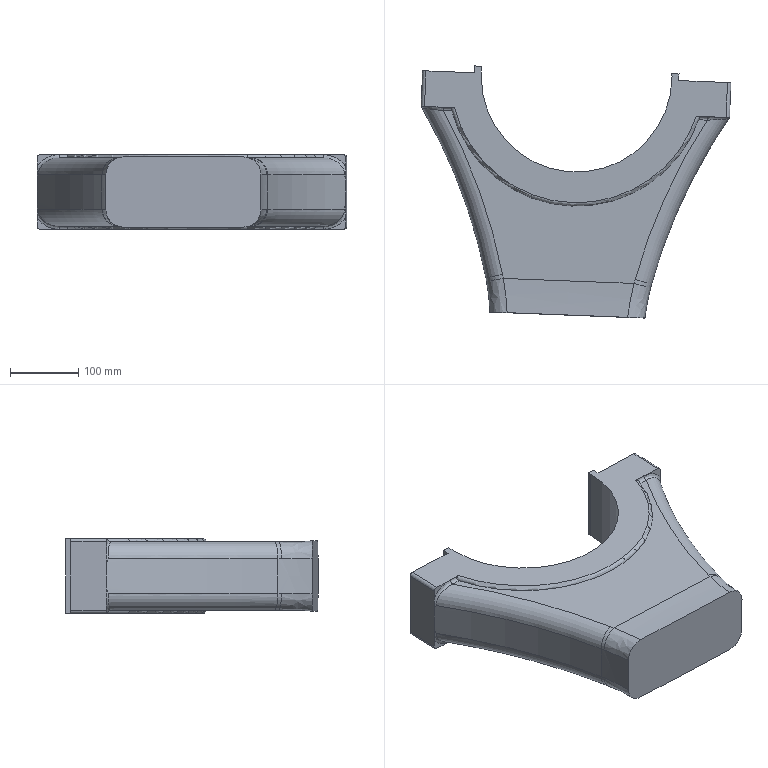Part | SolidWorks | features BaseBody 1 | 1 solid | 58 faces | box 455.294 x 369.863 x 110 mm | volume 8796602 mm3 | plane 19 | cylinder 17 | spline 16 | torus 6 | commonest cylinder face diameters 10 x8 20 x4 280 x3 1620 x2